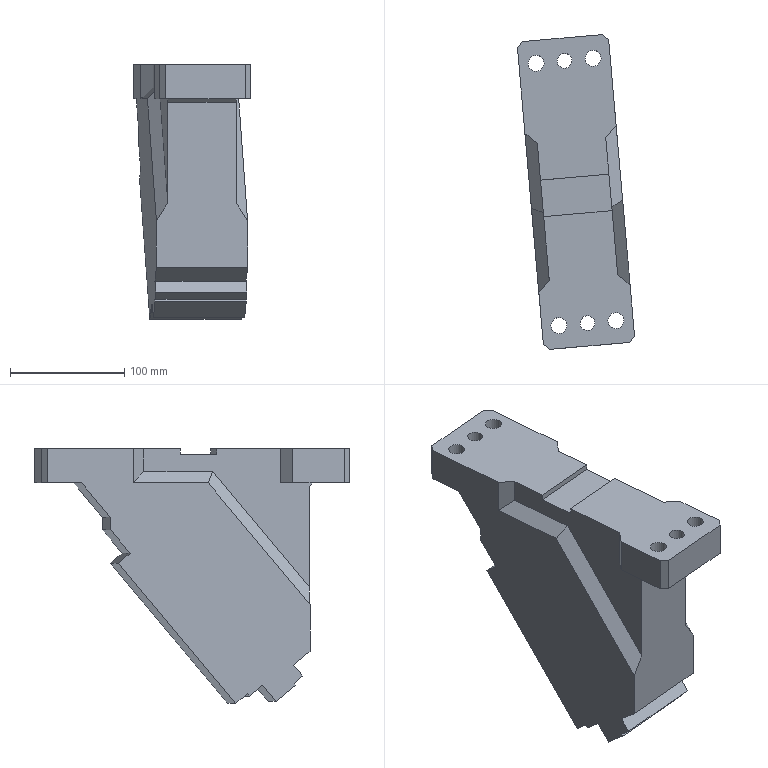Part | NX | features solid 2 | 1 solid | 57 faces | box 102.356 x 275.073 x 222.611 mm | volume 2513550 mm3 | plane 47 | cylinder 10 | commonest cylinder face diameters 14 x4 20 x4 13 x2